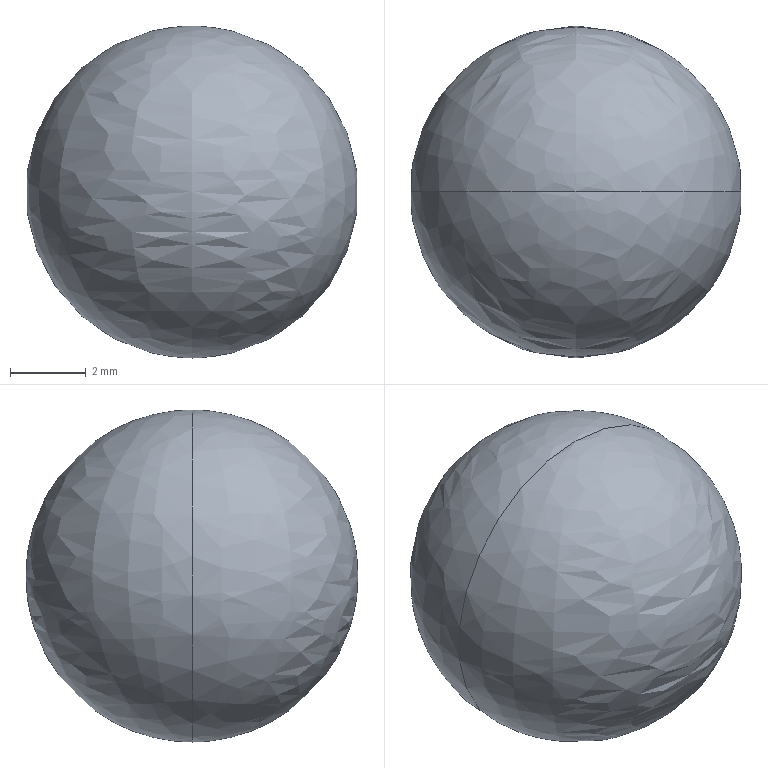Part | SolidWorks | features BaseBody 1 | 1 solid | 2 faces | volume 350.762 mm3 | spline 2